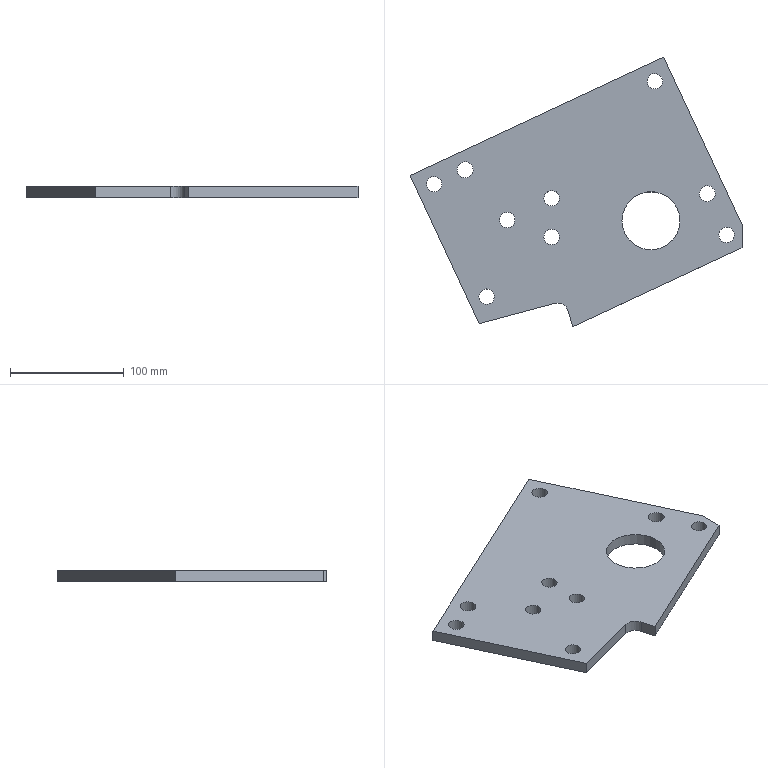Part | NX | features 6 2 | 1 solid | 20 faces | box 291.706 x 237.073 x 10 mm | volume 388045 mm3 | cylinder 11 | plane 9 | commonest cylinder face diameters 13.5 x7 14.001 x2 20 x1 51 x1
STEP:
#1=CARTESIAN_POINT('',(739.523,139.747,101.));
#2=VERTEX_POINT('',#1);
#3=CARTESIAN_POINT('',(732.773,139.747,101.));
#4=DIRECTION('',(0.,0.,1.));
#5=DIRECTION('',(1.,0.,0.));
#6=AXIS2_PLACEMENT_3D('',#3,#4,#5);
#7=CIRCLE('',#6,6.75);
#8=EDGE_CURVE('',#2,#2,#7,.T.);
#9=ORIENTED_EDGE('',*,*,#8,.F.);
#10=EDGE_LOOP('',(#9));
#11=FACE_BOUND('',#10,.T.);
#12=CARTESIAN_POINT('',(739.523,105.747,101.));
#13=VERTEX_POINT('',#12);
#14=CARTESIAN_POINT('',(732.773,105.747,101.));
#15=DIRECTION('',(0.,0.,1.));
#16=DIRECTION('',(1.,0.,0.));
#17=AXIS2_PLACEMENT_3D('',#14,#15,#16);
#18=CIRCLE('',#17,6.75);
#19=EDGE_CURVE('',#13,#13,#18,.T.);
#20=ORIENTED_EDGE('',*,*,#19,.F.);
#21=EDGE_LOOP('',(#20));
#22=FACE_BOUND('',#21,.T.);
#23=CARTESIAN_POINT('',(845.5,120.,101.));
#24=VERTEX_POINT('',#23);
#25=CARTESIAN_POINT('',(820.,120.,101.));
#26=DIRECTION('',(0.,0.,1.));
#27=DIRECTION('',(1.,0.,0.));
#28=AXIS2_PLACEMENT_3D('',#25,#26,#27);
#29=CIRCLE('',#28,25.5);
#30=EDGE_CURVE('',#24,#24,#29,.T.);
#31=ORIENTED_EDGE('',*,*,#30,.F.);
#32=EDGE_LOOP('',(#31));
#33=FACE_BOUND('',#32,.T.);
#34=CARTESIAN_POINT('',(872.53,137.451,101.));
#35=VERTEX_POINT('',#34);
#36=CARTESIAN_POINT('',(869.572,143.795,101.));
#37=DIRECTION('',(0.,0.,1.));
#38=DIRECTION('',(0.4226,-0.9063,0.));
#39=AXIS2_PLACEMENT_3D('',#36,#37,#38);
#40=CIRCLE('',#39,7.);
#41=EDGE_CURVE('',#35,#35,#40,.T.);
#42=ORIENTED_EDGE('',*,*,#41,.F.);
#43=EDGE_LOOP('',(#42));
#44=FACE_BOUND('',#43,.T.);
#45=CARTESIAN_POINT('',(681.739,56.208,101.));
#46=VERTEX_POINT('',#45);
#47=CARTESIAN_POINT('',(675.622,53.355,101.));
#48=DIRECTION('',(0.,0.,1.));
#49=DIRECTION('',(0.9063,0.4226,0.));
#50=AXIS2_PLACEMENT_3D('',#47,#48,#49);
#51=CIRCLE('',#50,6.75);
#52=EDGE_CURVE('',#46,#46,#51,.T.);
#53=ORIENTED_EDGE('',*,*,#52,.F.);
#54=EDGE_LOOP('',(#53));
#55=FACE_BOUND('',#54,.T.);
#56=CARTESIAN_POINT('',(892.594,110.396,101.));
#57=VERTEX_POINT('',#56);
#58=CARTESIAN_POINT('',(886.476,107.543,101.));
#59=DIRECTION('',(0.,0.,1.));
#60=DIRECTION('',(0.9063,0.4226,0.));
#61=AXIS2_PLACEMENT_3D('',#58,#59,#60);
#62=CIRCLE('',#61,6.75);
#63=EDGE_CURVE('',#57,#57,#62,.T.);
#64=ORIENTED_EDGE('',*,*,#63,.F.);
#65=EDGE_LOOP('',(#64));
#66=FACE_BOUND('',#65,.T.);
#67=CARTESIAN_POINT('',(635.674,154.995,101.));
#68=VERTEX_POINT('',#67);
#69=CARTESIAN_POINT('',(629.556,152.142,101.));
#70=DIRECTION('',(0.,0.,1.));
#71=DIRECTION('',(0.9063,0.4226,0.));
#72=AXIS2_PLACEMENT_3D('',#69,#70,#71);
#73=CIRCLE('',#72,6.75);
#74=EDGE_CURVE('',#68,#68,#73,.T.);
#75=ORIENTED_EDGE('',*,*,#74,.F.);
#76=EDGE_LOOP('',(#75));
#77=FACE_BOUND('',#76,.T.);
#78=CARTESIAN_POINT('',(829.624,245.435,101.));
#79=VERTEX_POINT('',#78);
#80=CARTESIAN_POINT('',(823.506,242.583,101.));
#81=DIRECTION('',(0.,0.,1.));
#82=DIRECTION('',(0.9063,0.4226,0.));
#83=AXIS2_PLACEMENT_3D('',#80,#81,#82);
#84=CIRCLE('',#83,6.75);
#85=EDGE_CURVE('',#79,#79,#84,.T.);
#86=ORIENTED_EDGE('',*,*,#85,.F.);
#87=EDGE_LOOP('',(#86));
#88=FACE_BOUND('',#87,.T.);
#89=CARTESIAN_POINT('',(663.09,167.779,101.));
#90=VERTEX_POINT('',#89);
#91=CARTESIAN_POINT('',(656.746,164.821,101.));
#92=DIRECTION('',(0.,0.,1.));
#93=DIRECTION('',(0.9063,0.4226,0.));
#94=AXIS2_PLACEMENT_3D('',#91,#92,#93);
#95=CIRCLE('',#94,7.);
#96=EDGE_CURVE('',#90,#90,#95,.T.);
#97=ORIENTED_EDGE('',*,*,#96,.F.);
#98=EDGE_LOOP('',(#97));
#99=FACE_BOUND('',#98,.T.);
#100=CARTESIAN_POINT('',(700.523,120.747,101.));
#101=VERTEX_POINT('',#100);
#102=CARTESIAN_POINT('',(693.773,120.747,101.));
#103=DIRECTION('',(0.,0.,-1.));
#104=DIRECTION('',(1.,0.,0.));
#105=AXIS2_PLACEMENT_3D('',#102,#103,#104);
#106=CIRCLE('',#105,6.75);
#107=EDGE_CURVE('',#101,#101,#106,.T.);
#108=ORIENTED_EDGE('',*,*,#107,.T.);
#109=EDGE_LOOP('',(#108));
#110=FACE_BOUND('',#109,.T.);
#111=CARTESIAN_POINT('',(751.123,26.773,101.));
#112=VERTEX_POINT('',#111);
#113=CARTESIAN_POINT('',(900.,96.195,101.));
#114=VERTEX_POINT('',#113);
#115=CARTESIAN_POINT('',(791.732,45.709,101.));
#116=DIRECTION('',(0.9063,0.4226,0.));
#117=VECTOR('',#116,1000.);
#118=LINE('',#115,#117);
#119=EDGE_CURVE('',#112,#114,#118,.T.);
#120=ORIENTED_EDGE('',*,*,#119,.T.);
#121=CARTESIAN_POINT('',(900.,116.401,101.));
#122=VERTEX_POINT('',#121);
#123=CARTESIAN_POINT('',(900.,-207.622,101.));
#124=DIRECTION('',(0.,1.,0.));
#125=VECTOR('',#124,1000.);
#126=LINE('',#123,#125);
#127=EDGE_CURVE('',#114,#122,#126,.T.);
#128=ORIENTED_EDGE('',*,*,#127,.T.);
#129=CARTESIAN_POINT('',(831.245,263.846,101.));
#130=VERTEX_POINT('',#129);
#131=CARTESIAN_POINT('',(861.04,199.951,101.));
#132=DIRECTION('',(-0.4226,0.9063,0.));
#133=VECTOR('',#132,1000.);
#134=LINE('',#131,#133);
#135=EDGE_CURVE('',#122,#130,#134,.T.);
#136=ORIENTED_EDGE('',*,*,#135,.T.);
#137=CARTESIAN_POINT('',(608.294,159.881,101.));
#138=VERTEX_POINT('',#137);
#139=CARTESIAN_POINT('',(715.238,209.75,101.));
#140=DIRECTION('',(-0.9063,-0.4226,0.));
#141=VECTOR('',#140,1000.);
#142=LINE('',#139,#141);
#143=EDGE_CURVE('',#130,#138,#142,.T.);
#144=ORIENTED_EDGE('',*,*,#143,.T.);
#145=CARTESIAN_POINT('',(669.005,29.685,101.));
#146=VERTEX_POINT('',#145);
#147=CARTESIAN_POINT('',(638.088,95.987,101.));
#148=DIRECTION('',(0.4226,-0.9063,0.));
#149=VECTOR('',#148,1000.);
#150=LINE('',#147,#149);
#151=EDGE_CURVE('',#138,#146,#150,.T.);
#152=ORIENTED_EDGE('',*,*,#151,.T.);
#153=CARTESIAN_POINT('',(735.235,47.431,101.));
#154=VERTEX_POINT('',#153);
#155=CARTESIAN_POINT('',(633.813,20.255,101.));
#156=DIRECTION('',(0.9659,0.2588,0.));
#157=VECTOR('',#156,1000.);
#158=LINE('',#155,#157);
#159=EDGE_CURVE('',#146,#154,#158,.T.);
#160=ORIENTED_EDGE('',*,*,#159,.T.);
#161=CARTESIAN_POINT('',(747.483,40.36,101.));
#162=VERTEX_POINT('',#161);
#163=CARTESIAN_POINT('',(737.823,37.772,101.));
#164=DIRECTION('',(0.,0.,-1.));
#165=DIRECTION('',(1.,0.,0.));
#166=AXIS2_PLACEMENT_3D('',#163,#164,#165);
#167=CIRCLE('',#166,10.);
#168=EDGE_CURVE('',#154,#162,#167,.T.);
#169=ORIENTED_EDGE('',*,*,#168,.T.);
#170=CARTESIAN_POINT('',(763.012,-17.595,101.));
#171=DIRECTION('',(0.2588,-0.9659,0.));
#172=VECTOR('',#171,1000.);
#173=LINE('',#170,#172);
#174=EDGE_CURVE('',#162,#112,#173,.T.);
#175=ORIENTED_EDGE('',*,*,#174,.T.);
#176=EDGE_LOOP('',(#120,#128,#136,#144,#152,#160,#169,#175));
#177=FACE_BOUND('',#176,.T.);
#178=CARTESIAN_POINT('',(615.919,-207.622,101.));
#179=DIRECTION('',(0.,0.,1.));
#180=DIRECTION('',(-0.9063,-0.4226,0.));
#181=AXIS2_PLACEMENT_3D('',#178,#179,#180);
#182=PLANE('',#181);
#183=ADVANCED_FACE('',(#11,#22,#33,#44,#55,#66,#77,#88,#99,#110,#177),#182,.T.);
#184=CARTESIAN_POINT('',(726.023,139.747,91.));
#185=VERTEX_POINT('',#184);
#186=CARTESIAN_POINT('',(732.773,139.747,91.));
#187=DIRECTION('',(0.,0.,-1.));
#188=DIRECTION('',(-1.,0.,0.));
#189=AXIS2_PLACEMENT_3D('',#186,#187,#188);
#190=CIRCLE('',#189,6.75);
#191=EDGE_CURVE('',#185,#185,#190,.T.);
#192=ORIENTED_EDGE('',*,*,#191,.F.);
#193=EDGE_LOOP('',(#192));
#194=FACE_BOUND('',#193,.T.);
#195=CARTESIAN_POINT('',(726.023,105.747,91.));
#196=VERTEX_POINT('',#195);
#197=CARTESIAN_POINT('',(732.773,105.747,91.));
#198=DIRECTION('',(0.,0.,1.));
#199=DIRECTION('',(-1.,0.,0.));
#200=AXIS2_PLACEMENT_3D('',#197,#198,#199);
#201=CIRCLE('',#200,6.75);
#202=EDGE_CURVE('',#196,#196,#201,.T.);
#203=ORIENTED_EDGE('',*,*,#202,.T.);
#204=EDGE_LOOP('',(#203));
#205=FACE_BOUND('',#204,.T.);
#206=CARTESIAN_POINT('',(794.5,120.,91.));
#207=VERTEX_POINT('',#206);
#208=CARTESIAN_POINT('',(820.,120.,91.));
#209=DIRECTION('',(0.,0.,1.));
#210=DIRECTION('',(-1.,0.,0.));
#211=AXIS2_PLACEMENT_3D('',#208,#209,#210);
#212=CIRCLE('',#211,25.5);
#213=EDGE_CURVE('',#207,#207,#212,.T.);
#214=ORIENTED_EDGE('',*,*,#213,.T.);
#215=EDGE_LOOP('',(#214));
#216=FACE_BOUND('',#215,.T.);
#217=CARTESIAN_POINT('',(872.53,137.451,91.));
#218=VERTEX_POINT('',#217);
#219=CARTESIAN_POINT('',(869.572,143.795,91.));
#220=DIRECTION('',(0.,0.,-1.));
#221=DIRECTION('',(0.4226,-0.9063,0.));
#222=AXIS2_PLACEMENT_3D('',#219,#220,#221);
#223=CIRCLE('',#222,7.);
#224=EDGE_CURVE('',#218,#218,#223,.T.);
#225=ORIENTED_EDGE('',*,*,#224,.F.);
#226=EDGE_LOOP('',(#225));
#227=FACE_BOUND('',#226,.T.);
#228=CARTESIAN_POINT('',(681.739,56.208,91.));
#229=VERTEX_POINT('',#228);
#230=CARTESIAN_POINT('',(675.622,53.355,91.));
#231=DIRECTION('',(0.,0.,-1.));
#232=DIRECTION('',(0.9063,0.4226,0.));
#233=AXIS2_PLACEMENT_3D('',#230,#231,#232);
#234=CIRCLE('',#233,6.75);
#235=EDGE_CURVE('',#229,#229,#234,.T.);
#236=ORIENTED_EDGE('',*,*,#235,.F.);
#237=EDGE_LOOP('',(#236));
#238=FACE_BOUND('',#237,.T.);
#239=CARTESIAN_POINT('',(892.594,110.396,91.));
#240=VERTEX_POINT('',#239);
#241=CARTESIAN_POINT('',(886.476,107.543,91.));
#242=DIRECTION('',(0.,0.,-1.));
#243=DIRECTION('',(0.9063,0.4226,0.));
#244=AXIS2_PLACEMENT_3D('',#241,#242,#243);
#245=CIRCLE('',#244,6.75);
#246=EDGE_CURVE('',#240,#240,#245,.T.);
#247=ORIENTED_EDGE('',*,*,#246,.F.);
#248=EDGE_LOOP('',(#247));
#249=FACE_BOUND('',#248,.T.);
#250=CARTESIAN_POINT('',(635.674,154.995,91.));
#251=VERTEX_POINT('',#250);
#252=CARTESIAN_POINT('',(629.556,152.142,91.));
#253=DIRECTION('',(0.,0.,-1.));
#254=DIRECTION('',(0.9063,0.4226,0.));
#255=AXIS2_PLACEMENT_3D('',#252,#253,#254);
#256=CIRCLE('',#255,6.75);
#257=EDGE_CURVE('',#251,#251,#256,.T.);
#258=ORIENTED_EDGE('',*,*,#257,.F.);
#259=EDGE_LOOP('',(#258));
#260=FACE_BOUND('',#259,.T.);
#261=CARTESIAN_POINT('',(829.624,245.435,91.));
#262=VERTEX_POINT('',#261);
#263=CARTESIAN_POINT('',(823.506,242.583,91.));
#264=DIRECTION('',(0.,0.,-1.));
#265=DIRECTION('',(0.9063,0.4226,0.));
#266=AXIS2_PLACEMENT_3D('',#263,#264,#265);
#267=CIRCLE('',#266,6.75);
#268=EDGE_CURVE('',#262,#262,#267,.T.);
#269=ORIENTED_EDGE('',*,*,#268,.F.);
#270=EDGE_LOOP('',(#269));
#271=FACE_BOUND('',#270,.T.);
#272=CARTESIAN_POINT('',(663.09,167.779,91.));
#273=VERTEX_POINT('',#272);
#274=CARTESIAN_POINT('',(656.746,164.821,91.));
#275=DIRECTION('',(0.,0.,-1.));
#276=DIRECTION('',(0.9063,0.4226,0.));
#277=AXIS2_PLACEMENT_3D('',#274,#275,#276);
#278=CIRCLE('',#277,7.);
#279=EDGE_CURVE('',#273,#273,#278,.T.);
#280=ORIENTED_EDGE('',*,*,#279,.F.);
#281=EDGE_LOOP('',(#280));
#282=FACE_BOUND('',#281,.T.);
#283=CARTESIAN_POINT('',(687.023,120.747,91.));
#284=VERTEX_POINT('',#283);
#285=CARTESIAN_POINT('',(693.773,120.747,91.));
#286=DIRECTION('',(0.,0.,-1.));
#287=DIRECTION('',(-1.,0.,0.));
#288=AXIS2_PLACEMENT_3D('',#285,#286,#287);
#289=CIRCLE('',#288,6.75);
#290=EDGE_CURVE('',#284,#284,#289,.T.);
#291=ORIENTED_EDGE('',*,*,#290,.F.);
#292=EDGE_LOOP('',(#291));
#293=FACE_BOUND('',#292,.T.);
#294=CARTESIAN_POINT('',(831.245,263.846,91.));
#295=VERTEX_POINT('',#294);
#296=CARTESIAN_POINT('',(900.,116.401,91.));
#297=VERTEX_POINT('',#296);
#298=CARTESIAN_POINT('',(861.04,199.951,91.));
#299=DIRECTION('',(0.4226,-0.9063,0.));
#300=VECTOR('',#299,1000.);
#301=LINE('',#298,#300);
#302=EDGE_CURVE('',#295,#297,#301,.T.);
#303=ORIENTED_EDGE('',*,*,#302,.T.);
#304=CARTESIAN_POINT('',(900.,96.195,91.));
#305=VERTEX_POINT('',#304);
#306=CARTESIAN_POINT('',(900.,145.856,91.));
#307=DIRECTION('',(0.,-1.,0.));
#308=VECTOR('',#307,1000.);
#309=LINE('',#306,#308);
#310=EDGE_CURVE('',#297,#305,#309,.T.);
#311=ORIENTED_EDGE('',*,*,#310,.T.);
#312=CARTESIAN_POINT('',(751.123,26.773,91.));
#313=VERTEX_POINT('',#312);
#314=CARTESIAN_POINT('',(791.732,45.709,91.));
#315=DIRECTION('',(-0.9063,-0.4226,0.));
#316=VECTOR('',#315,1000.);
#317=LINE('',#314,#316);
#318=EDGE_CURVE('',#305,#313,#317,.T.);
#319=ORIENTED_EDGE('',*,*,#318,.T.);
#320=CARTESIAN_POINT('',(747.483,40.36,91.));
#321=VERTEX_POINT('',#320);
#322=CARTESIAN_POINT('',(763.012,-17.595,91.));
#323=DIRECTION('',(-0.2588,0.9659,0.));
#324=VECTOR('',#323,1000.);
#325=LINE('',#322,#324);
#326=EDGE_CURVE('',#313,#321,#325,.T.);
#327=ORIENTED_EDGE('',*,*,#326,.T.);
#328=CARTESIAN_POINT('',(735.235,47.431,91.));
#329=VERTEX_POINT('',#328);
#330=CARTESIAN_POINT('',(737.823,37.772,91.));
#331=DIRECTION('',(0.,0.,1.));
#332=DIRECTION('',(-1.,0.,0.));
#333=AXIS2_PLACEMENT_3D('',#330,#331,#332);
#334=CIRCLE('',#333,10.);
#335=EDGE_CURVE('',#321,#329,#334,.T.);
#336=ORIENTED_EDGE('',*,*,#335,.T.);
#337=CARTESIAN_POINT('',(669.005,29.685,91.));
#338=VERTEX_POINT('',#337);
#339=CARTESIAN_POINT('',(633.813,20.255,91.));
#340=DIRECTION('',(-0.9659,-0.2588,0.));
#341=VECTOR('',#340,1000.);
#342=LINE('',#339,#341);
#343=EDGE_CURVE('',#329,#338,#342,.T.);
#344=ORIENTED_EDGE('',*,*,#343,.T.);
#345=CARTESIAN_POINT('',(608.294,159.881,91.));
#346=VERTEX_POINT('',#345);
#347=CARTESIAN_POINT('',(638.088,95.987,91.));
#348=DIRECTION('',(-0.4226,0.9063,0.));
#349=VECTOR('',#348,1000.);
#350=LINE('',#347,#349);
#351=EDGE_CURVE('',#338,#346,#350,.T.);
#352=ORIENTED_EDGE('',*,*,#351,.T.);
#353=CARTESIAN_POINT('',(715.238,209.75,91.));
#354=DIRECTION('',(0.9063,0.4226,0.));
#355=VECTOR('',#354,1000.);
#356=LINE('',#353,#355);
#357=EDGE_CURVE('',#346,#295,#356,.T.);
#358=ORIENTED_EDGE('',*,*,#357,.T.);
#359=EDGE_LOOP('',(#303,#311,#319,#327,#336,#344,#352,#358));
#360=FACE_BOUND('',#359,.T.);
#361=CARTESIAN_POINT('',(745.033,145.856,91.));
#362=DIRECTION('',(0.,0.,-1.));
#363=DIRECTION('',(0.9063,0.4226,0.));
#364=AXIS2_PLACEMENT_3D('',#361,#362,#363);
#365=PLANE('',#364);
#366=ADVANCED_FACE('',(#194,#205,#216,#227,#238,#249,#260,#271,#282,#293,#360),#365,.T.);
#367=ORIENTED_EDGE('',*,*,#318,.F.);
#368=CARTESIAN_POINT('',(900.,96.195,91.));
#369=DIRECTION('',(0.,0.,1.));
#370=VECTOR('',#369,1000.);
#371=LINE('',#368,#370);
#372=EDGE_CURVE('',#305,#114,#371,.T.);
#373=ORIENTED_EDGE('',*,*,#372,.T.);
#374=ORIENTED_EDGE('',*,*,#119,.F.);
#375=CARTESIAN_POINT('',(751.123,26.773,91.));
#376=DIRECTION('',(0.,0.,1.));
#377=VECTOR('',#376,1000.);
#378=LINE('',#375,#377);
#379=EDGE_CURVE('',#313,#112,#378,.T.);
#380=ORIENTED_EDGE('',*,*,#379,.F.);
#381=EDGE_LOOP('',(#367,#373,#374,#380));
#382=FACE_BOUND('',#381,.T.);
#383=CARTESIAN_POINT('',(791.732,45.709,91.));
#384=DIRECTION('',(0.4226,-0.9063,0.));
#385=DIRECTION('',(0.,0.,-1.));
#386=AXIS2_PLACEMENT_3D('',#383,#384,#385);
#387=PLANE('',#386);
#388=ADVANCED_FACE('',(#382),#387,.T.);
#389=ORIENTED_EDGE('',*,*,#135,.F.);
#390=CARTESIAN_POINT('',(900.,116.401,91.));
#391=DIRECTION('',(0.,0.,-1.));
#392=VECTOR('',#391,1000.);
#393=LINE('',#390,#392);
#394=EDGE_CURVE('',#122,#297,#393,.T.);
#395=ORIENTED_EDGE('',*,*,#394,.T.);
#396=ORIENTED_EDGE('',*,*,#302,.F.);
#397=CARTESIAN_POINT('',(831.245,263.846,91.));
#398=DIRECTION('',(0.,0.,1.));
#399=VECTOR('',#398,1000.);
#400=LINE('',#397,#399);
#401=EDGE_CURVE('',#295,#130,#400,.T.);
#402=ORIENTED_EDGE('',*,*,#401,.T.);
#403=EDGE_LOOP('',(#389,#395,#396,#402));
#404=FACE_BOUND('',#403,.T.);
#405=CARTESIAN_POINT('',(861.04,199.951,91.));
#406=DIRECTION('',(0.9063,0.4226,0.));
#407=DIRECTION('',(0.,0.,1.));
#408=AXIS2_PLACEMENT_3D('',#405,#406,#407);
#409=PLANE('',#408);
#410=ADVANCED_FACE('',(#404),#409,.T.);
#411=ORIENTED_EDGE('',*,*,#401,.F.);
#412=ORIENTED_EDGE('',*,*,#357,.F.);
#413=CARTESIAN_POINT('',(608.294,159.881,91.));
#414=DIRECTION('',(0.,0.,1.));
#415=VECTOR('',#414,1000.);
#416=LINE('',#413,#415);
#417=EDGE_CURVE('',#346,#138,#416,.T.);
#418=ORIENTED_EDGE('',*,*,#417,.T.);
#419=ORIENTED_EDGE('',*,*,#143,.F.);
#420=EDGE_LOOP('',(#411,#412,#418,#419));
#421=FACE_BOUND('',#420,.T.);
#422=CARTESIAN_POINT('',(715.238,209.75,91.));
#423=DIRECTION('',(-0.4226,0.9063,0.));
#424=DIRECTION('',(0.,0.,1.));
#425=AXIS2_PLACEMENT_3D('',#422,#423,#424);
#426=PLANE('',#425);
#427=ADVANCED_FACE('',(#421),#426,.T.);
#428=CARTESIAN_POINT('',(669.005,29.685,91.));
#429=DIRECTION('',(0.,0.,-1.));
#430=VECTOR('',#429,1000.);
#431=LINE('',#428,#430);
#432=EDGE_CURVE('',#146,#338,#431,.T.);
#433=ORIENTED_EDGE('',*,*,#432,.F.);
#434=ORIENTED_EDGE('',*,*,#151,.F.);
#435=ORIENTED_EDGE('',*,*,#417,.F.);
#436=ORIENTED_EDGE('',*,*,#351,.F.);
#437=EDGE_LOOP('',(#433,#434,#435,#436));
#438=FACE_BOUND('',#437,.T.);
#439=CARTESIAN_POINT('',(638.088,95.987,91.));
#440=DIRECTION('',(-0.9063,-0.4226,0.));
#441=DIRECTION('',(0.,0.,-1.));
#442=AXIS2_PLACEMENT_3D('',#439,#440,#441);
#443=PLANE('',#442);
#444=ADVANCED_FACE('',(#438),#443,.T.);
#445=ORIENTED_EDGE('',*,*,#74,.T.);
#446=EDGE_LOOP('',(#445));
#447=FACE_BOUND('',#446,.T.);
#448=ORIENTED_EDGE('',*,*,#257,.T.);
#449=EDGE_LOOP('',(#448));
#450=FACE_BOUND('',#449,.T.);
#451=CARTESIAN_POINT('',(629.556,152.142,91.));
#452=DIRECTION('',(0.,0.,1.));
#453=DIRECTION('',(-0.9063,-0.4226,0.));
#454=AXIS2_PLACEMENT_3D('',#451,#452,#453);
#455=CYLINDRICAL_SURFACE('',#454,6.75);
#456=ADVANCED_FACE('',(#447,#450),#455,.F.);
#457=ORIENTED_EDGE('',*,*,#63,.T.);
#458=EDGE_LOOP('',(#457));
#459=FACE_BOUND('',#458,.T.);
#460=ORIENTED_EDGE('',*,*,#246,.T.);
#461=EDGE_LOOP('',(#460));
#462=FACE_BOUND('',#461,.T.);
#463=CARTESIAN_POINT('',(886.476,107.543,91.));
#464=DIRECTION('',(0.,0.,1.));
#465=DIRECTION('',(-0.9063,-0.4226,0.));
#466=AXIS2_PLACEMENT_3D('',#463,#464,#465);
#467=CYLINDRICAL_SURFACE('',#466,6.75);
#468=ADVANCED_FACE('',(#459,#462),#467,.F.);
#469=ORIENTED_EDGE('',*,*,#85,.T.);
#470=EDGE_LOOP('',(#469));
#471=FACE_BOUND('',#470,.T.);
#472=ORIENTED_EDGE('',*,*,#268,.T.);
#473=EDGE_LOOP('',(#472));
#474=FACE_BOUND('',#473,.T.);
#475=CARTESIAN_POINT('',(823.506,242.583,91.));
#476=DIRECTION('',(0.,0.,1.));
#477=DIRECTION('',(-0.9063,-0.4226,0.));
#478=AXIS2_PLACEMENT_3D('',#475,#476,#477);
#479=CYLINDRICAL_SURFACE('',#478,6.75);
#480=ADVANCED_FACE('',(#471,#474),#479,.F.);
#481=ORIENTED_EDGE('',*,*,#52,.T.);
#482=EDGE_LOOP('',(#481));
#483=FACE_BOUND('',#482,.T.);
#484=ORIENTED_EDGE('',*,*,#235,.T.);
#485=EDGE_LOOP('',(#484));
#486=FACE_BOUND('',#485,.T.);
#487=CARTESIAN_POINT('',(675.622,53.355,91.));
#488=DIRECTION('',(0.,0.,1.));
#489=DIRECTION('',(-0.9063,-0.4226,0.));
#490=AXIS2_PLACEMENT_3D('',#487,#488,#489);
#491=CYLINDRICAL_SURFACE('',#490,6.75);
#492=ADVANCED_FACE('',(#483,#486),#491,.F.);
#493=ORIENTED_EDGE('',*,*,#96,.T.);
#494=EDGE_LOOP('',(#493));
#495=FACE_BOUND('',#494,.T.);
#496=ORIENTED_EDGE('',*,*,#279,.T.);
#497=EDGE_LOOP('',(#496));
#498=FACE_BOUND('',#497,.T.);
#499=CARTESIAN_POINT('',(656.746,164.821,91.));
#500=DIRECTION('',(0.,0.,1.));
#501=DIRECTION('',(-0.9063,-0.4226,0.));
#502=AXIS2_PLACEMENT_3D('',#499,#500,#501);
#503=CYLINDRICAL_SURFACE('',#502,7.);
#504=ADVANCED_FACE('',(#495,#498),#503,.F.);
#505=ORIENTED_EDGE('',*,*,#41,.T.);
#506=EDGE_LOOP('',(#505));
#507=FACE_BOUND('',#506,.T.);
#508=ORIENTED_EDGE('',*,*,#224,.T.);
#509=EDGE_LOOP('',(#508));
#510=FACE_BOUND('',#509,.T.);
#511=CARTESIAN_POINT('',(869.572,143.795,91.));
#512=DIRECTION('',(0.,0.,1.));
#513=DIRECTION('',(-0.4226,0.9063,0.));
#514=AXIS2_PLACEMENT_3D('',#511,#512,#513);
#515=CYLINDRICAL_SURFACE('',#514,7.);
#516=ADVANCED_FACE('',(#507,#510),#515,.F.);
#517=ORIENTED_EDGE('',*,*,#343,.F.);
#518=CARTESIAN_POINT('',(735.235,47.431,101.));
#519=DIRECTION('',(0.,0.,1.));
#520=VECTOR('',#519,1000.);
#521=LINE('',#518,#520);
#522=EDGE_CURVE('',#329,#154,#521,.T.);
#523=ORIENTED_EDGE('',*,*,#522,.T.);
#524=ORIENTED_EDGE('',*,*,#159,.F.);
#525=ORIENTED_EDGE('',*,*,#432,.T.);
#526=EDGE_LOOP('',(#517,#523,#524,#525));
#527=FACE_BOUND('',#526,.T.);
#528=CARTESIAN_POINT('',(633.813,20.255,91.));
#529=DIRECTION('',(-0.2588,0.9659,0.));
#530=DIRECTION('',(0.,0.,-1.));
#531=AXIS2_PLACEMENT_3D('',#528,#529,#530);
#532=PLANE('',#531);
#533=ADVANCED_FACE('',(#527),#532,.F.);
#534=ORIENTED_EDGE('',*,*,#174,.F.);
#535=CARTESIAN_POINT('',(747.483,40.36,91.));
#536=DIRECTION('',(0.,0.,-1.));
#537=VECTOR('',#536,1000.);
#538=LINE('',#535,#537);
#539=EDGE_CURVE('',#162,#321,#538,.T.);
#540=ORIENTED_EDGE('',*,*,#539,.T.);
#541=ORIENTED_EDGE('',*,*,#326,.F.);
#542=ORIENTED_EDGE('',*,*,#379,.T.);
#543=EDGE_LOOP('',(#534,#540,#541,#542));
#544=FACE_BOUND('',#543,.T.);
#545=CARTESIAN_POINT('',(763.012,-17.595,91.));
#546=DIRECTION('',(0.9659,0.2588,0.));
#547=DIRECTION('',(0.,0.,1.));
#548=AXIS2_PLACEMENT_3D('',#545,#546,#547);
#549=PLANE('',#548);
#550=ADVANCED_FACE('',(#544),#549,.F.);
#551=ORIENTED_EDGE('',*,*,#168,.F.);
#552=ORIENTED_EDGE('',*,*,#522,.F.);
#553=ORIENTED_EDGE('',*,*,#335,.F.);
#554=ORIENTED_EDGE('',*,*,#539,.F.);
#555=EDGE_LOOP('',(#551,#552,#553,#554));
#556=FACE_BOUND('',#555,.T.);
#557=CARTESIAN_POINT('',(737.823,37.772,91.));
#558=DIRECTION('',(0.,0.,1.));
#559=DIRECTION('',(-1.,0.,0.));
#560=AXIS2_PLACEMENT_3D('',#557,#558,#559);
#561=CYLINDRICAL_SURFACE('',#560,10.);
#562=ADVANCED_FACE('',(#556),#561,.F.);
#563=ORIENTED_EDGE('',*,*,#30,.T.);
#564=EDGE_LOOP('',(#563));
#565=FACE_BOUND('',#564,.T.);
#566=ORIENTED_EDGE('',*,*,#213,.F.);
#567=EDGE_LOOP('',(#566));
#568=FACE_BOUND('',#567,.T.);
#569=CARTESIAN_POINT('',(820.,120.,-83.));
#570=DIRECTION('',(0.,0.,1.));
#571=DIRECTION('',(-1.,0.,0.));
#572=AXIS2_PLACEMENT_3D('',#569,#570,#571);
#573=CYLINDRICAL_SURFACE('',#572,25.5);
#574=ADVANCED_FACE('',(#565,#568),#573,.F.);
#575=ORIENTED_EDGE('',*,*,#19,.T.);
#576=EDGE_LOOP('',(#575));
#577=FACE_BOUND('',#576,.T.);
#578=ORIENTED_EDGE('',*,*,#202,.F.);
#579=EDGE_LOOP('',(#578));
#580=FACE_BOUND('',#579,.T.);
#581=CARTESIAN_POINT('',(732.773,105.747,-61.));
#582=DIRECTION('',(0.,0.,1.));
#583=DIRECTION('',(-1.,0.,0.));
#584=AXIS2_PLACEMENT_3D('',#581,#582,#583);
#585=CYLINDRICAL_SURFACE('',#584,6.75);
#586=ADVANCED_FACE('',(#577,#580),#585,.F.);
#587=ORIENTED_EDGE('',*,*,#107,.F.);
#588=EDGE_LOOP('',(#587));
#589=FACE_BOUND('',#588,.T.);
#590=ORIENTED_EDGE('',*,*,#290,.T.);
#591=EDGE_LOOP('',(#590));
#592=FACE_BOUND('',#591,.T.);
#593=CARTESIAN_POINT('',(693.773,120.747,-61.));
#594=DIRECTION('',(0.,0.,1.));
#595=DIRECTION('',(-1.,0.,0.));
#596=AXIS2_PLACEMENT_3D('',#593,#594,#595);
#597=CYLINDRICAL_SURFACE('',#596,6.75);
#598=ADVANCED_FACE('',(#589,#592),#597,.F.);
#599=ORIENTED_EDGE('',*,*,#8,.T.);
#600=EDGE_LOOP('',(#599));
#601=FACE_BOUND('',#600,.T.);
#602=ORIENTED_EDGE('',*,*,#191,.T.);
#603=EDGE_LOOP('',(#602));
#604=FACE_BOUND('',#603,.T.);
#605=CARTESIAN_POINT('',(732.773,139.747,-61.));
#606=DIRECTION('',(0.,0.,1.));
#607=DIRECTION('',(-1.,0.,0.));
#608=AXIS2_PLACEMENT_3D('',#605,#606,#607);
#609=CYLINDRICAL_SURFACE('',#608,6.75);
#610=ADVANCED_FACE('',(#601,#604),#609,.F.);
#611=ORIENTED_EDGE('',*,*,#372,.F.);
#612=ORIENTED_EDGE('',*,*,#310,.F.);
#613=ORIENTED_EDGE('',*,*,#394,.F.);
#614=ORIENTED_EDGE('',*,*,#127,.F.);
#615=EDGE_LOOP('',(#611,#612,#613,#614));
#616=FACE_BOUND('',#615,.T.);
#617=CARTESIAN_POINT('',(900.,32.5,30.));
#618=DIRECTION('',(1.,0.,0.));
#619=DIRECTION('',(0.,0.,1.));
#620=AXIS2_PLACEMENT_3D('',#617,#618,#619);
#621=PLANE('',#620);
#622=ADVANCED_FACE('',(#616),#621,.T.);
#623=CLOSED_SHELL('',(#183,#366,#388,#410,#427,#444,#456,#468,#480,#492,#504,#516,#533,#550,#562,#574,#586,#598,#610,#622));
#624=MANIFOLD_SOLID_BREP('',#623);
#625=(LENGTH_UNIT()NAMED_UNIT(*)SI_UNIT(.MILLI.,.METRE.));
#626=UNCERTAINTY_MEASURE_WITH_UNIT(LENGTH_MEASURE(0.00001),#625,'','');
#627=(NAMED_UNIT(*)PLANE_ANGLE_UNIT()SI_UNIT($,.RADIAN.));
#628=(NAMED_UNIT(*)SI_UNIT($,.STERADIAN.)SOLID_ANGLE_UNIT());
#629=(GEOMETRIC_REPRESENTATION_CONTEXT(3)GLOBAL_UNCERTAINTY_ASSIGNED_CONTEXT((#626))GLOBAL_UNIT_ASSIGNED_CONTEXT((#625,#627,#628))REPRESENTATION_CONTEXT('',''));
#630=ADVANCED_BREP_SHAPE_REPRESENTATION('',(#624),#629);